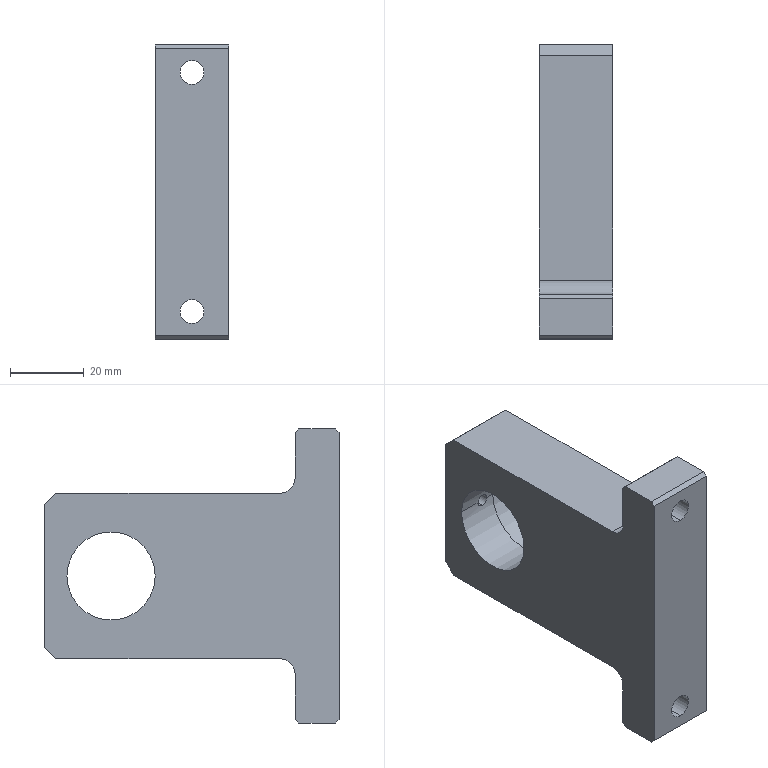Part | STEP file | Small support plate A | 1 solid | 45 faces | box 20 x 80 x 80 mm | volume 68710 mm3 | cylinder 20 | plane 17 | cone 8 | commonest cylinder face diameters 3.3 x10 6.5 x4 8 x2 24 x2 28 x2